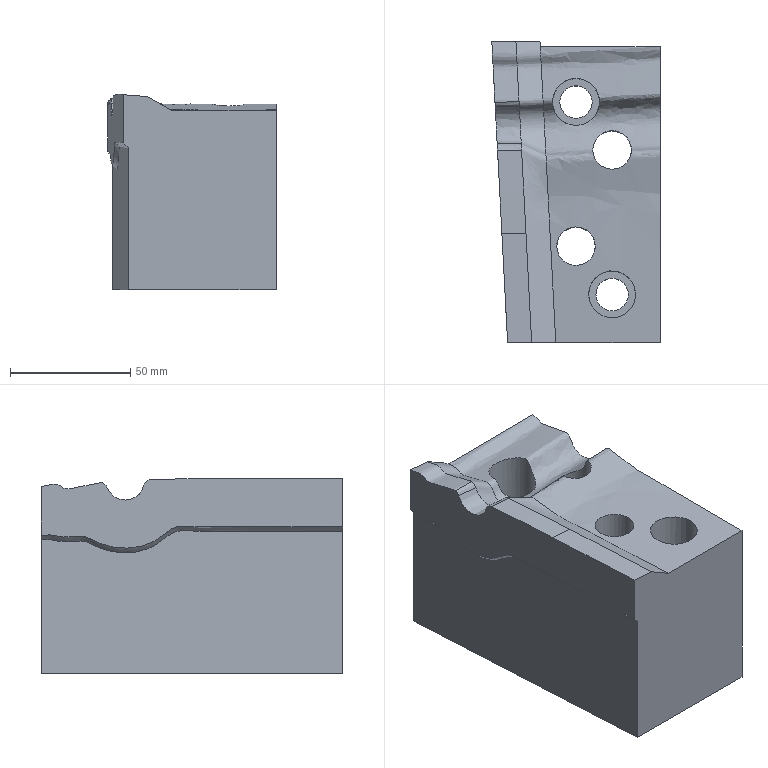Part | NX | features solid 2 | 1 solid | 25 faces | box 70.001 x 125.701 x 81.279 mm | volume 530163 mm3 | spline 10 | plane 9 | cylinder 6 | commonest cylinder face diameters 13.5 x2 16 x2 19.5 x2